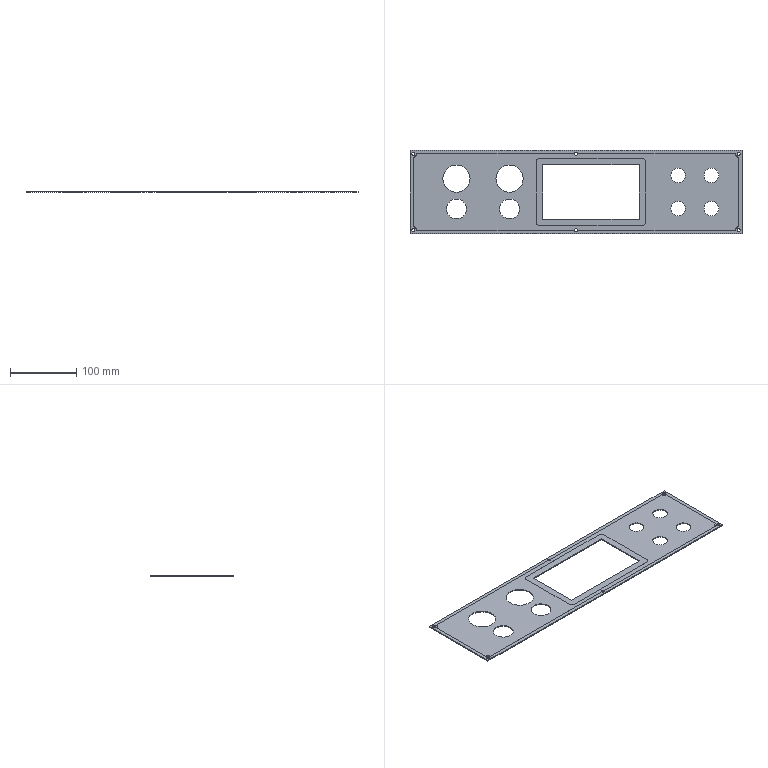Part | STEP file | Panel | 1 solid | 58 faces | box 500 x 125 x 1.5 mm | volume 67047 mm3 | cylinder 36 | plane 22 | commonest cylinder face diameters 5 x12 10 x8 22 x8 30 x4 41 x4